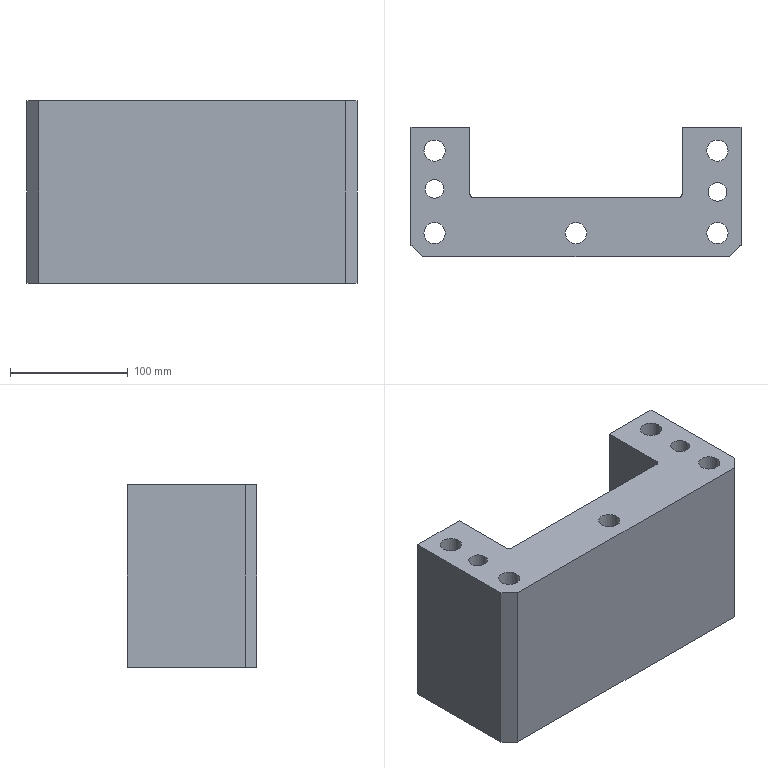Part | NX | features FD 2 | 1 solid | 47 faces | box 280 x 110 x 155 mm | volume 2587040 mm3 | plane 23 | cylinder 22 | cone 2 | commonest cylinder face diameters 18 x5 26 x5 21 x4 6 x2 14.1 x2 16.001 x2
STEP:
#1=CARTESIAN_POINT('',(2683.,562.5,256.5));
#2=VERTEX_POINT('',#1);
#3=CARTESIAN_POINT('',(2943.,562.5,256.5));
#4=VERTEX_POINT('',#3);
#5=CARTESIAN_POINT('',(2738.,562.5,256.5));
#6=DIRECTION('',(1.,0.,0.));
#7=VECTOR('',#6,1000.);
#8=LINE('',#5,#7);
#9=EDGE_CURVE('',#2,#4,#8,.T.);
#10=ORIENTED_EDGE('',*,*,#9,.F.);
#11=CARTESIAN_POINT('',(2683.,562.5,101.5));
#12=VERTEX_POINT('',#11);
#13=CARTESIAN_POINT('',(2683.,562.5,101.5));
#14=DIRECTION('',(0.,0.,-1.));
#15=VECTOR('',#14,1000.);
#16=LINE('',#13,#15);
#17=EDGE_CURVE('',#2,#12,#16,.T.);
#18=ORIENTED_EDGE('',*,*,#17,.T.);
#19=CARTESIAN_POINT('',(2943.,562.5,101.5));
#20=VERTEX_POINT('',#19);
#21=CARTESIAN_POINT('',(2738.,562.5,101.5));
#22=DIRECTION('',(1.,0.,0.));
#23=VECTOR('',#22,1000.);
#24=LINE('',#21,#23);
#25=EDGE_CURVE('',#12,#20,#24,.T.);
#26=ORIENTED_EDGE('',*,*,#25,.T.);
#27=CARTESIAN_POINT('',(2943.,562.5,191.5));
#28=DIRECTION('',(0.,0.,1.));
#29=VECTOR('',#28,1000.);
#30=LINE('',#27,#29);
#31=EDGE_CURVE('',#20,#4,#30,.T.);
#32=ORIENTED_EDGE('',*,*,#31,.T.);
#33=EDGE_LOOP('',(#10,#18,#26,#32));
#34=FACE_BOUND('',#33,.T.);
#35=CARTESIAN_POINT('',(2738.,562.5,191.5));
#36=DIRECTION('',(0.,1.,0.));
#37=DIRECTION('',(1.,0.,0.));
#38=AXIS2_PLACEMENT_3D('',#35,#36,#37);
#39=PLANE('',#38);
#40=ADVANCED_FACE('',(#34),#39,.F.);
#41=CARTESIAN_POINT('',(2953.,572.5,256.5));
#42=VERTEX_POINT('',#41);
#43=CARTESIAN_POINT('',(2953.,672.5,256.5));
#44=VERTEX_POINT('',#43);
#45=CARTESIAN_POINT('',(2953.,622.5,256.5));
#46=DIRECTION('',(0.,1.,0.));
#47=VECTOR('',#46,1000.);
#48=LINE('',#45,#47);
#49=EDGE_CURVE('',#42,#44,#48,.T.);
#50=ORIENTED_EDGE('',*,*,#49,.F.);
#51=CARTESIAN_POINT('',(2953.,572.5,101.5));
#52=VERTEX_POINT('',#51);
#53=CARTESIAN_POINT('',(2953.,572.5,191.5));
#54=DIRECTION('',(0.,0.,-1.));
#55=VECTOR('',#54,1000.);
#56=LINE('',#53,#55);
#57=EDGE_CURVE('',#42,#52,#56,.T.);
#58=ORIENTED_EDGE('',*,*,#57,.T.);
#59=CARTESIAN_POINT('',(2953.,672.5,101.5));
#60=VERTEX_POINT('',#59);
#61=CARTESIAN_POINT('',(2953.,622.5,101.5));
#62=DIRECTION('',(0.,1.,0.));
#63=VECTOR('',#62,1000.);
#64=LINE('',#61,#63);
#65=EDGE_CURVE('',#52,#60,#64,.T.);
#66=ORIENTED_EDGE('',*,*,#65,.T.);
#67=CARTESIAN_POINT('',(2953.,672.5,191.5));
#68=DIRECTION('',(0.,0.,1.));
#69=VECTOR('',#68,1000.);
#70=LINE('',#67,#69);
#71=EDGE_CURVE('',#60,#44,#70,.T.);
#72=ORIENTED_EDGE('',*,*,#71,.T.);
#73=EDGE_LOOP('',(#50,#58,#66,#72));
#74=FACE_BOUND('',#73,.T.);
#75=CARTESIAN_POINT('',(2953.,622.5,191.5));
#76=DIRECTION('',(-1.,0.,0.));
#77=DIRECTION('',(0.,1.,0.));
#78=AXIS2_PLACEMENT_3D('',#75,#76,#77);
#79=PLANE('',#78);
#80=ADVANCED_FACE('',(#74),#79,.F.);
#81=ORIENTED_EDGE('',*,*,#71,.F.);
#82=CARTESIAN_POINT('',(2903.,672.5,101.5));
#83=VERTEX_POINT('',#82);
#84=CARTESIAN_POINT('',(2918.,672.5,101.5));
#85=DIRECTION('',(1.,0.,0.));
#86=VECTOR('',#85,1000.);
#87=LINE('',#84,#86);
#88=EDGE_CURVE('',#83,#60,#87,.T.);
#89=ORIENTED_EDGE('',*,*,#88,.F.);
#90=CARTESIAN_POINT('',(2903.,672.5,256.5));
#91=VERTEX_POINT('',#90);
#92=CARTESIAN_POINT('',(2903.,672.5,191.5));
#93=DIRECTION('',(0.,0.,1.));
#94=VECTOR('',#93,1000.);
#95=LINE('',#92,#94);
#96=EDGE_CURVE('',#83,#91,#95,.T.);
#97=ORIENTED_EDGE('',*,*,#96,.T.);
#98=CARTESIAN_POINT('',(2918.,672.5,256.5));
#99=DIRECTION('',(1.,0.,0.));
#100=VECTOR('',#99,1000.);
#101=LINE('',#98,#100);
#102=EDGE_CURVE('',#91,#44,#101,.T.);
#103=ORIENTED_EDGE('',*,*,#102,.T.);
#104=EDGE_LOOP('',(#81,#89,#97,#103));
#105=FACE_BOUND('',#104,.T.);
#106=CARTESIAN_POINT('',(2918.,672.5,191.5));
#107=DIRECTION('',(0.,-1.,0.));
#108=DIRECTION('',(-1.,0.,0.));
#109=AXIS2_PLACEMENT_3D('',#106,#107,#108);
#110=PLANE('',#109);
#111=ADVANCED_FACE('',(#105),#110,.F.);
#112=CARTESIAN_POINT('',(2903.,615.5,101.5));
#113=VERTEX_POINT('',#112);
#114=CARTESIAN_POINT('',(2903.,622.5,101.5));
#115=DIRECTION('',(0.,1.,0.));
#116=VECTOR('',#115,1000.);
#117=LINE('',#114,#116);
#118=EDGE_CURVE('',#113,#83,#117,.T.);
#119=ORIENTED_EDGE('',*,*,#118,.F.);
#120=CARTESIAN_POINT('',(2903.,615.5,256.5));
#121=VERTEX_POINT('',#120);
#122=CARTESIAN_POINT('',(2903.,615.5,191.5));
#123=DIRECTION('',(0.,0.,1.));
#124=VECTOR('',#123,1000.);
#125=LINE('',#122,#124);
#126=EDGE_CURVE('',#113,#121,#125,.T.);
#127=ORIENTED_EDGE('',*,*,#126,.T.);
#128=CARTESIAN_POINT('',(2903.,622.5,256.5));
#129=DIRECTION('',(0.,1.,0.));
#130=VECTOR('',#129,1000.);
#131=LINE('',#128,#130);
#132=EDGE_CURVE('',#121,#91,#131,.T.);
#133=ORIENTED_EDGE('',*,*,#132,.T.);
#134=ORIENTED_EDGE('',*,*,#96,.F.);
#135=EDGE_LOOP('',(#119,#127,#133,#134));
#136=FACE_BOUND('',#135,.T.);
#137=CARTESIAN_POINT('',(2903.,622.5,191.5));
#138=DIRECTION('',(1.,0.,0.));
#139=DIRECTION('',(0.,-1.,0.));
#140=AXIS2_PLACEMENT_3D('',#137,#138,#139);
#141=PLANE('',#140);
#142=ADVANCED_FACE('',(#136),#141,.F.);
#143=CARTESIAN_POINT('',(2900.,612.5,101.5));
#144=VERTEX_POINT('',#143);
#145=CARTESIAN_POINT('',(2900.,615.5,101.5));
#146=DIRECTION('',(0.,0.,1.));
#147=DIRECTION('',(-1.,0.,0.));
#148=AXIS2_PLACEMENT_3D('',#145,#146,#147);
#149=CIRCLE('',#148,3.);
#150=EDGE_CURVE('',#144,#113,#149,.T.);
#151=ORIENTED_EDGE('',*,*,#150,.F.);
#152=CARTESIAN_POINT('',(2900.,612.5,256.5));
#153=VERTEX_POINT('',#152);
#154=CARTESIAN_POINT('',(2900.,612.5,191.5));
#155=DIRECTION('',(0.,0.,-1.));
#156=VECTOR('',#155,1000.);
#157=LINE('',#154,#156);
#158=EDGE_CURVE('',#153,#144,#157,.T.);
#159=ORIENTED_EDGE('',*,*,#158,.F.);
#160=CARTESIAN_POINT('',(2900.,615.5,256.5));
#161=DIRECTION('',(0.,0.,-1.));
#162=DIRECTION('',(1.,0.,0.));
#163=AXIS2_PLACEMENT_3D('',#160,#161,#162);
#164=CIRCLE('',#163,3.);
#165=EDGE_CURVE('',#121,#153,#164,.T.);
#166=ORIENTED_EDGE('',*,*,#165,.F.);
#167=ORIENTED_EDGE('',*,*,#126,.F.);
#168=EDGE_LOOP('',(#151,#159,#166,#167));
#169=FACE_BOUND('',#168,.T.);
#170=CARTESIAN_POINT('',(2900.,615.5,191.5));
#171=DIRECTION('',(0.,0.,-1.));
#172=DIRECTION('',(-1.,0.,0.));
#173=AXIS2_PLACEMENT_3D('',#170,#171,#172);
#174=CYLINDRICAL_SURFACE('',#173,3.);
#175=ADVANCED_FACE('',(#169),#174,.F.);
#176=CARTESIAN_POINT('',(2883.5,612.5,226.5));
#177=VERTEX_POINT('',#176);
#178=CARTESIAN_POINT('',(2873.,612.5,226.5));
#179=DIRECTION('',(0.,-1.,0.));
#180=DIRECTION('',(1.,0.,0.));
#181=AXIS2_PLACEMENT_3D('',#178,#179,#180);
#182=CIRCLE('',#181,10.5);
#183=EDGE_CURVE('',#177,#177,#182,.T.);
#184=ORIENTED_EDGE('',*,*,#183,.T.);
#185=EDGE_LOOP('',(#184));
#186=FACE_BOUND('',#185,.T.);
#187=CARTESIAN_POINT('',(2763.5,612.5,226.5));
#188=VERTEX_POINT('',#187);
#189=CARTESIAN_POINT('',(2753.,612.5,226.5));
#190=DIRECTION('',(0.,-1.,0.));
#191=DIRECTION('',(1.,0.,0.));
#192=AXIS2_PLACEMENT_3D('',#189,#190,#191);
#193=CIRCLE('',#192,10.5);
#194=EDGE_CURVE('',#188,#188,#193,.T.);
#195=ORIENTED_EDGE('',*,*,#194,.T.);
#196=EDGE_LOOP('',(#195));
#197=FACE_BOUND('',#196,.T.);
#198=CARTESIAN_POINT('',(2763.5,612.5,134.));
#199=VERTEX_POINT('',#198);
#200=CARTESIAN_POINT('',(2753.,612.5,134.));
#201=DIRECTION('',(0.,-1.,0.));
#202=DIRECTION('',(1.,0.,0.));
#203=AXIS2_PLACEMENT_3D('',#200,#201,#202);
#204=CIRCLE('',#203,10.5);
#205=EDGE_CURVE('',#199,#199,#204,.T.);
#206=ORIENTED_EDGE('',*,*,#205,.T.);
#207=EDGE_LOOP('',(#206));
#208=FACE_BOUND('',#207,.T.);
#209=CARTESIAN_POINT('',(2883.5,612.5,134.));
#210=VERTEX_POINT('',#209);
#211=CARTESIAN_POINT('',(2873.,612.5,134.));
#212=DIRECTION('',(0.,-1.,0.));
#213=DIRECTION('',(1.,0.,0.));
#214=AXIS2_PLACEMENT_3D('',#211,#212,#213);
#215=CIRCLE('',#214,10.5);
#216=EDGE_CURVE('',#210,#210,#215,.T.);
#217=ORIENTED_EDGE('',*,*,#216,.T.);
#218=EDGE_LOOP('',(#217));
#219=FACE_BOUND('',#218,.T.);
#220=CARTESIAN_POINT('',(2726.,612.5,101.5));
#221=VERTEX_POINT('',#220);
#222=CARTESIAN_POINT('',(2738.,612.5,101.5));
#223=DIRECTION('',(1.,0.,0.));
#224=VECTOR('',#223,1000.);
#225=LINE('',#222,#224);
#226=EDGE_CURVE('',#221,#144,#225,.T.);
#227=ORIENTED_EDGE('',*,*,#226,.F.);
#228=CARTESIAN_POINT('',(2726.,612.5,256.5));
#229=VERTEX_POINT('',#228);
#230=CARTESIAN_POINT('',(2726.,612.5,191.5));
#231=DIRECTION('',(0.,0.,1.));
#232=VECTOR('',#231,1000.);
#233=LINE('',#230,#232);
#234=EDGE_CURVE('',#221,#229,#233,.T.);
#235=ORIENTED_EDGE('',*,*,#234,.T.);
#236=CARTESIAN_POINT('',(2738.,612.5,256.5));
#237=DIRECTION('',(1.,0.,0.));
#238=VECTOR('',#237,1000.);
#239=LINE('',#236,#238);
#240=EDGE_CURVE('',#229,#153,#239,.T.);
#241=ORIENTED_EDGE('',*,*,#240,.T.);
#242=ORIENTED_EDGE('',*,*,#158,.T.);
#243=EDGE_LOOP('',(#227,#235,#241,#242));
#244=FACE_BOUND('',#243,.T.);
#245=CARTESIAN_POINT('',(2738.,612.5,191.5));
#246=DIRECTION('',(0.,-1.,0.));
#247=DIRECTION('',(-1.,0.,0.));
#248=AXIS2_PLACEMENT_3D('',#245,#246,#247);
#249=PLANE('',#248);
#250=ADVANCED_FACE('',(#186,#197,#208,#219,#244),#249,.F.);
#251=CARTESIAN_POINT('',(2723.,615.5,101.5));
#252=VERTEX_POINT('',#251);
#253=CARTESIAN_POINT('',(2726.,615.5,101.5));
#254=DIRECTION('',(0.,0.,1.));
#255=DIRECTION('',(-1.,0.,0.));
#256=AXIS2_PLACEMENT_3D('',#253,#254,#255);
#257=CIRCLE('',#256,3.);
#258=EDGE_CURVE('',#252,#221,#257,.T.);
#259=ORIENTED_EDGE('',*,*,#258,.F.);
#260=CARTESIAN_POINT('',(2723.,615.5,256.5));
#261=VERTEX_POINT('',#260);
#262=CARTESIAN_POINT('',(2723.,615.5,191.5));
#263=DIRECTION('',(0.,0.,-1.));
#264=VECTOR('',#263,1000.);
#265=LINE('',#262,#264);
#266=EDGE_CURVE('',#261,#252,#265,.T.);
#267=ORIENTED_EDGE('',*,*,#266,.F.);
#268=CARTESIAN_POINT('',(2726.,615.5,256.5));
#269=DIRECTION('',(0.,0.,-1.));
#270=DIRECTION('',(1.,0.,0.));
#271=AXIS2_PLACEMENT_3D('',#268,#269,#270);
#272=CIRCLE('',#271,3.);
#273=EDGE_CURVE('',#229,#261,#272,.T.);
#274=ORIENTED_EDGE('',*,*,#273,.F.);
#275=ORIENTED_EDGE('',*,*,#234,.F.);
#276=EDGE_LOOP('',(#259,#267,#274,#275));
#277=FACE_BOUND('',#276,.T.);
#278=CARTESIAN_POINT('',(2726.,615.5,191.5));
#279=DIRECTION('',(0.,0.,-1.));
#280=DIRECTION('',(-1.,0.,0.));
#281=AXIS2_PLACEMENT_3D('',#278,#279,#280);
#282=CYLINDRICAL_SURFACE('',#281,3.);
#283=ADVANCED_FACE('',(#277),#282,.F.);
#284=CARTESIAN_POINT('',(2723.,672.5,256.5));
#285=VERTEX_POINT('',#284);
#286=CARTESIAN_POINT('',(2723.,667.5,256.5));
#287=DIRECTION('',(0.,-1.,0.));
#288=VECTOR('',#287,1000.);
#289=LINE('',#286,#288);
#290=EDGE_CURVE('',#285,#261,#289,.T.);
#291=ORIENTED_EDGE('',*,*,#290,.T.);
#292=ORIENTED_EDGE('',*,*,#266,.T.);
#293=CARTESIAN_POINT('',(2723.,672.5,101.5));
#294=VERTEX_POINT('',#293);
#295=CARTESIAN_POINT('',(2723.,667.5,101.5));
#296=DIRECTION('',(0.,-1.,0.));
#297=VECTOR('',#296,1000.);
#298=LINE('',#295,#297);
#299=EDGE_CURVE('',#294,#252,#298,.T.);
#300=ORIENTED_EDGE('',*,*,#299,.F.);
#301=CARTESIAN_POINT('',(2723.,672.5,191.5));
#302=DIRECTION('',(0.,0.,1.));
#303=VECTOR('',#302,1000.);
#304=LINE('',#301,#303);
#305=EDGE_CURVE('',#294,#285,#304,.T.);
#306=ORIENTED_EDGE('',*,*,#305,.T.);
#307=EDGE_LOOP('',(#291,#292,#300,#306));
#308=FACE_BOUND('',#307,.T.);
#309=CARTESIAN_POINT('',(2723.,667.5,191.5));
#310=DIRECTION('',(-1.,0.,0.));
#311=DIRECTION('',(0.,1.,0.));
#312=AXIS2_PLACEMENT_3D('',#309,#310,#311);
#313=PLANE('',#312);
#314=ADVANCED_FACE('',(#308),#313,.F.);
#315=ORIENTED_EDGE('',*,*,#305,.F.);
#316=CARTESIAN_POINT('',(2673.,672.5,101.5));
#317=VERTEX_POINT('',#316);
#318=CARTESIAN_POINT('',(2708.,672.5,101.5));
#319=DIRECTION('',(-1.,0.,0.));
#320=VECTOR('',#319,1000.);
#321=LINE('',#318,#320);
#322=EDGE_CURVE('',#294,#317,#321,.T.);
#323=ORIENTED_EDGE('',*,*,#322,.T.);
#324=CARTESIAN_POINT('',(2673.,672.5,256.5));
#325=VERTEX_POINT('',#324);
#326=CARTESIAN_POINT('',(2673.,672.5,191.5));
#327=DIRECTION('',(0.,0.,1.));
#328=VECTOR('',#327,1000.);
#329=LINE('',#326,#328);
#330=EDGE_CURVE('',#317,#325,#329,.T.);
#331=ORIENTED_EDGE('',*,*,#330,.T.);
#332=CARTESIAN_POINT('',(2708.,672.5,256.5));
#333=DIRECTION('',(-1.,0.,0.));
#334=VECTOR('',#333,1000.);
#335=LINE('',#332,#334);
#336=EDGE_CURVE('',#285,#325,#335,.T.);
#337=ORIENTED_EDGE('',*,*,#336,.F.);
#338=EDGE_LOOP('',(#315,#323,#331,#337));
#339=FACE_BOUND('',#338,.T.);
#340=CARTESIAN_POINT('',(2708.,672.5,191.5));
#341=DIRECTION('',(0.,1.,0.));
#342=DIRECTION('',(1.,0.,0.));
#343=AXIS2_PLACEMENT_3D('',#340,#341,#342);
#344=PLANE('',#343);
#345=ADVANCED_FACE('',(#339),#344,.T.);
#346=CARTESIAN_POINT('',(2673.,572.5,101.5));
#347=VERTEX_POINT('',#346);
#348=CARTESIAN_POINT('',(2673.,667.5,101.5));
#349=DIRECTION('',(0.,-1.,0.));
#350=VECTOR('',#349,1000.);
#351=LINE('',#348,#350);
#352=EDGE_CURVE('',#317,#347,#351,.T.);
#353=ORIENTED_EDGE('',*,*,#352,.T.);
#354=CARTESIAN_POINT('',(2673.,572.5,256.5));
#355=VERTEX_POINT('',#354);
#356=CARTESIAN_POINT('',(2673.,572.5,276.5));
#357=DIRECTION('',(0.,0.,1.));
#358=VECTOR('',#357,1000.);
#359=LINE('',#356,#358);
#360=EDGE_CURVE('',#347,#355,#359,.T.);
#361=ORIENTED_EDGE('',*,*,#360,.T.);
#362=CARTESIAN_POINT('',(2673.,667.5,256.5));
#363=DIRECTION('',(0.,-1.,0.));
#364=VECTOR('',#363,1000.);
#365=LINE('',#362,#364);
#366=EDGE_CURVE('',#325,#355,#365,.T.);
#367=ORIENTED_EDGE('',*,*,#366,.F.);
#368=ORIENTED_EDGE('',*,*,#330,.F.);
#369=EDGE_LOOP('',(#353,#361,#367,#368));
#370=FACE_BOUND('',#369,.T.);
#371=CARTESIAN_POINT('',(2673.,667.5,191.5));
#372=DIRECTION('',(-1.,0.,0.));
#373=DIRECTION('',(0.,1.,0.));
#374=AXIS2_PLACEMENT_3D('',#371,#372,#373);
#375=PLANE('',#374);
#376=ADVANCED_FACE('',(#370),#375,.T.);
#377=CARTESIAN_POINT('',(2701.001,620.,256.5));
#378=VERTEX_POINT('',#377);
#379=CARTESIAN_POINT('',(2693.,620.,256.5));
#380=DIRECTION('',(0.,0.,-1.));
#381=DIRECTION('',(1.,0.,0.));
#382=AXIS2_PLACEMENT_3D('',#379,#380,#381);
#383=CIRCLE('',#382,8.001);
#384=EDGE_CURVE('',#378,#378,#383,.T.);
#385=ORIENTED_EDGE('',*,*,#384,.T.);
#386=EDGE_LOOP('',(#385));
#387=FACE_BOUND('',#386,.T.);
#388=CARTESIAN_POINT('',(2941.001,617.5,256.5));
#389=VERTEX_POINT('',#388);
#390=CARTESIAN_POINT('',(2933.,617.5,256.5));
#391=DIRECTION('',(0.,0.,-1.));
#392=DIRECTION('',(1.,0.,0.));
#393=AXIS2_PLACEMENT_3D('',#390,#391,#392);
#394=CIRCLE('',#393,8.001);
#395=EDGE_CURVE('',#389,#389,#394,.T.);
#396=ORIENTED_EDGE('',*,*,#395,.T.);
#397=EDGE_LOOP('',(#396));
#398=FACE_BOUND('',#397,.T.);
#399=CARTESIAN_POINT('',(2822.,582.5,256.5));
#400=VERTEX_POINT('',#399);
#401=CARTESIAN_POINT('',(2813.,582.5,256.5));
#402=DIRECTION('',(0.,0.,-1.));
#403=DIRECTION('',(1.,0.,0.));
#404=AXIS2_PLACEMENT_3D('',#401,#402,#403);
#405=CIRCLE('',#404,9.);
#406=EDGE_CURVE('',#400,#400,#405,.T.);
#407=ORIENTED_EDGE('',*,*,#406,.T.);
#408=EDGE_LOOP('',(#407));
#409=FACE_BOUND('',#408,.T.);
#410=CARTESIAN_POINT('',(2942.,652.5,256.5));
#411=VERTEX_POINT('',#410);
#412=CARTESIAN_POINT('',(2933.,652.5,256.5));
#413=DIRECTION('',(0.,0.,-1.));
#414=DIRECTION('',(1.,0.,0.));
#415=AXIS2_PLACEMENT_3D('',#412,#413,#414);
#416=CIRCLE('',#415,9.);
#417=EDGE_CURVE('',#411,#411,#416,.T.);
#418=ORIENTED_EDGE('',*,*,#417,.T.);
#419=EDGE_LOOP('',(#418));
#420=FACE_BOUND('',#419,.T.);
#421=CARTESIAN_POINT('',(2702.,582.5,256.5));
#422=VERTEX_POINT('',#421);
#423=CARTESIAN_POINT('',(2693.,582.5,256.5));
#424=DIRECTION('',(0.,0.,-1.));
#425=DIRECTION('',(1.,0.,0.));
#426=AXIS2_PLACEMENT_3D('',#423,#424,#425);
#427=CIRCLE('',#426,9.);
#428=EDGE_CURVE('',#422,#422,#427,.T.);
#429=ORIENTED_EDGE('',*,*,#428,.T.);
#430=EDGE_LOOP('',(#429));
#431=FACE_BOUND('',#430,.T.);
#432=CARTESIAN_POINT('',(2702.,652.5,256.5));
#433=VERTEX_POINT('',#432);
#434=CARTESIAN_POINT('',(2693.,652.5,256.5));
#435=DIRECTION('',(0.,0.,-1.));
#436=DIRECTION('',(1.,0.,0.));
#437=AXIS2_PLACEMENT_3D('',#434,#435,#436);
#438=CIRCLE('',#437,9.);
#439=EDGE_CURVE('',#433,#433,#438,.T.);
#440=ORIENTED_EDGE('',*,*,#439,.T.);
#441=EDGE_LOOP('',(#440));
#442=FACE_BOUND('',#441,.T.);
#443=CARTESIAN_POINT('',(2942.,582.5,256.5));
#444=VERTEX_POINT('',#443);
#445=CARTESIAN_POINT('',(2933.,582.5,256.5));
#446=DIRECTION('',(0.,0.,-1.));
#447=DIRECTION('',(1.,0.,0.));
#448=AXIS2_PLACEMENT_3D('',#445,#446,#447);
#449=CIRCLE('',#448,9.);
#450=EDGE_CURVE('',#444,#444,#449,.T.);
#451=ORIENTED_EDGE('',*,*,#450,.T.);
#452=EDGE_LOOP('',(#451));
#453=FACE_BOUND('',#452,.T.);
#454=ORIENTED_EDGE('',*,*,#366,.T.);
#455=CARTESIAN_POINT('',(2658.,587.5,256.5));
#456=DIRECTION('',(0.7071,-0.7071,0.));
#457=VECTOR('',#456,1000.);
#458=LINE('',#455,#457);
#459=EDGE_CURVE('',#355,#2,#458,.T.);
#460=ORIENTED_EDGE('',*,*,#459,.T.);
#461=ORIENTED_EDGE('',*,*,#9,.T.);
#462=CARTESIAN_POINT('',(2893.,512.5,256.5));
#463=DIRECTION('',(0.7071,0.7071,0.));
#464=VECTOR('',#463,1000.);
#465=LINE('',#462,#464);
#466=EDGE_CURVE('',#4,#42,#465,.T.);
#467=ORIENTED_EDGE('',*,*,#466,.T.);
#468=ORIENTED_EDGE('',*,*,#49,.T.);
#469=ORIENTED_EDGE('',*,*,#102,.F.);
#470=ORIENTED_EDGE('',*,*,#132,.F.);
#471=ORIENTED_EDGE('',*,*,#165,.T.);
#472=ORIENTED_EDGE('',*,*,#240,.F.);
#473=ORIENTED_EDGE('',*,*,#273,.T.);
#474=ORIENTED_EDGE('',*,*,#290,.F.);
#475=ORIENTED_EDGE('',*,*,#336,.T.);
#476=EDGE_LOOP('',(#454,#460,#461,#467,#468,#469,#470,#471,#472,#473,#474,#475));
#477=FACE_BOUND('',#476,.T.);
#478=CARTESIAN_POINT('',(2738.,667.5,256.5));
#479=DIRECTION('',(0.,0.,1.));
#480=DIRECTION('',(0.,1.,0.));
#481=AXIS2_PLACEMENT_3D('',#478,#479,#480);
#482=PLANE('',#481);
#483=ADVANCED_FACE('',(#387,#398,#409,#420,#431,#442,#453,#477),#482,.T.);
#484=ORIENTED_EDGE('',*,*,#450,.F.);
#485=EDGE_LOOP('',(#484));
#486=FACE_BOUND('',#485,.T.);
#487=CARTESIAN_POINT('',(2942.,582.5,216.5));
#488=VERTEX_POINT('',#487);
#489=CARTESIAN_POINT('',(2933.,582.5,216.5));
#490=DIRECTION('',(0.,0.,-1.));
#491=DIRECTION('',(1.,0.,0.));
#492=AXIS2_PLACEMENT_3D('',#489,#490,#491);
#493=CIRCLE('',#492,9.);
#494=EDGE_CURVE('',#488,#488,#493,.T.);
#495=ORIENTED_EDGE('',*,*,#494,.T.);
#496=EDGE_LOOP('',(#495));
#497=FACE_BOUND('',#496,.T.);
#498=CARTESIAN_POINT('',(2933.,582.5,101.5));
#499=DIRECTION('',(0.,0.,1.));
#500=DIRECTION('',(1.,0.,0.));
#501=AXIS2_PLACEMENT_3D('',#498,#499,#500);
#502=CYLINDRICAL_SURFACE('',#501,9.);
#503=ADVANCED_FACE('',(#486,#497),#502,.F.);
#504=ORIENTED_EDGE('',*,*,#494,.F.);
#505=EDGE_LOOP('',(#504));
#506=FACE_BOUND('',#505,.T.);
#507=CARTESIAN_POINT('',(2946.,582.5,216.5));
#508=VERTEX_POINT('',#507);
#509=CARTESIAN_POINT('',(2933.,582.5,216.5));
#510=DIRECTION('',(0.,0.,-1.));
#511=DIRECTION('',(1.,0.,0.));
#512=AXIS2_PLACEMENT_3D('',#509,#510,#511);
#513=CIRCLE('',#512,13.);
#514=EDGE_CURVE('',#508,#508,#513,.T.);
#515=ORIENTED_EDGE('',*,*,#514,.T.);
#516=EDGE_LOOP('',(#515));
#517=FACE_BOUND('',#516,.T.);
#518=CARTESIAN_POINT('',(2933.,582.5,216.5));
#519=DIRECTION('',(0.,0.,1.));
#520=DIRECTION('',(1.,0.,0.));
#521=AXIS2_PLACEMENT_3D('',#518,#519,#520);
#522=PLANE('',#521);
#523=ADVANCED_FACE('',(#506,#517),#522,.F.);
#524=ORIENTED_EDGE('',*,*,#514,.F.);
#525=EDGE_LOOP('',(#524));
#526=FACE_BOUND('',#525,.T.);
#527=CARTESIAN_POINT('',(2946.,582.5,101.5));
#528=VERTEX_POINT('',#527);
#529=CARTESIAN_POINT('',(2933.,582.5,101.5));
#530=DIRECTION('',(0.,0.,-1.));
#531=DIRECTION('',(1.,0.,0.));
#532=AXIS2_PLACEMENT_3D('',#529,#530,#531);
#533=CIRCLE('',#532,13.);
#534=EDGE_CURVE('',#528,#528,#533,.T.);
#535=ORIENTED_EDGE('',*,*,#534,.T.);
#536=EDGE_LOOP('',(#535));
#537=FACE_BOUND('',#536,.T.);
#538=CARTESIAN_POINT('',(2933.,582.5,126.5));
#539=DIRECTION('',(0.,0.,1.));
#540=DIRECTION('',(1.,0.,0.));
#541=AXIS2_PLACEMENT_3D('',#538,#539,#540);
#542=CYLINDRICAL_SURFACE('',#541,13.);
#543=ADVANCED_FACE('',(#526,#537),#542,.F.);
#544=ORIENTED_EDGE('',*,*,#439,.F.);
#545=EDGE_LOOP('',(#544));
#546=FACE_BOUND('',#545,.T.);
#547=CARTESIAN_POINT('',(2702.,652.5,216.5));
#548=VERTEX_POINT('',#547);
#549=CARTESIAN_POINT('',(2693.,652.5,216.5));
#550=DIRECTION('',(0.,0.,-1.));
#551=DIRECTION('',(1.,0.,0.));
#552=AXIS2_PLACEMENT_3D('',#549,#550,#551);
#553=CIRCLE('',#552,9.);
#554=EDGE_CURVE('',#548,#548,#553,.T.);
#555=ORIENTED_EDGE('',*,*,#554,.T.);
#556=EDGE_LOOP('',(#555));
#557=FACE_BOUND('',#556,.T.);
#558=CARTESIAN_POINT('',(2693.,652.5,101.5));
#559=DIRECTION('',(0.,0.,1.));
#560=DIRECTION('',(1.,0.,0.));
#561=AXIS2_PLACEMENT_3D('',#558,#559,#560);
#562=CYLINDRICAL_SURFACE('',#561,9.);
#563=ADVANCED_FACE('',(#546,#557),#562,.F.);
#564=ORIENTED_EDGE('',*,*,#554,.F.);
#565=EDGE_LOOP('',(#564));
#566=FACE_BOUND('',#565,.T.);
#567=CARTESIAN_POINT('',(2706.,652.5,216.5));
#568=VERTEX_POINT('',#567);
#569=CARTESIAN_POINT('',(2693.,652.5,216.5));
#570=DIRECTION('',(0.,0.,-1.));
#571=DIRECTION('',(1.,0.,0.));
#572=AXIS2_PLACEMENT_3D('',#569,#570,#571);
#573=CIRCLE('',#572,13.);
#574=EDGE_CURVE('',#568,#568,#573,.T.);
#575=ORIENTED_EDGE('',*,*,#574,.T.);
#576=EDGE_LOOP('',(#575));
#577=FACE_BOUND('',#576,.T.);
#578=CARTESIAN_POINT('',(2693.,652.5,216.5));
#579=DIRECTION('',(0.,0.,1.));
#580=DIRECTION('',(1.,0.,0.));
#581=AXIS2_PLACEMENT_3D('',#578,#579,#580);
#582=PLANE('',#581);
#583=ADVANCED_FACE('',(#566,#577),#582,.F.);
#584=ORIENTED_EDGE('',*,*,#574,.F.);
#585=EDGE_LOOP('',(#584));
#586=FACE_BOUND('',#585,.T.);
#587=CARTESIAN_POINT('',(2706.,652.5,101.5));
#588=VERTEX_POINT('',#587);
#589=CARTESIAN_POINT('',(2693.,652.5,101.5));
#590=DIRECTION('',(0.,0.,-1.));
#591=DIRECTION('',(1.,0.,0.));
#592=AXIS2_PLACEMENT_3D('',#589,#590,#591);
#593=CIRCLE('',#592,13.);
#594=EDGE_CURVE('',#588,#588,#593,.T.);
#595=ORIENTED_EDGE('',*,*,#594,.T.);
#596=EDGE_LOOP('',(#595));
#597=FACE_BOUND('',#596,.T.);
#598=CARTESIAN_POINT('',(2693.,652.5,126.5));
#599=DIRECTION('',(0.,0.,1.));
#600=DIRECTION('',(1.,0.,0.));
#601=AXIS2_PLACEMENT_3D('',#598,#599,#600);
#602=CYLINDRICAL_SURFACE('',#601,13.);
#603=ADVANCED_FACE('',(#586,#597),#602,.F.);
#604=ORIENTED_EDGE('',*,*,#428,.F.);
#605=EDGE_LOOP('',(#604));
#606=FACE_BOUND('',#605,.T.);
#607=CARTESIAN_POINT('',(2702.,582.5,216.5));
#608=VERTEX_POINT('',#607);
#609=CARTESIAN_POINT('',(2693.,582.5,216.5));
#610=DIRECTION('',(0.,0.,-1.));
#611=DIRECTION('',(1.,0.,0.));
#612=AXIS2_PLACEMENT_3D('',#609,#610,#611);
#613=CIRCLE('',#612,9.);
#614=EDGE_CURVE('',#608,#608,#613,.T.);
#615=ORIENTED_EDGE('',*,*,#614,.T.);
#616=EDGE_LOOP('',(#615));
#617=FACE_BOUND('',#616,.T.);
#618=CARTESIAN_POINT('',(2693.,582.5,101.5));
#619=DIRECTION('',(0.,0.,1.));
#620=DIRECTION('',(1.,0.,0.));
#621=AXIS2_PLACEMENT_3D('',#618,#619,#620);
#622=CYLINDRICAL_SURFACE('',#621,9.);
#623=ADVANCED_FACE('',(#606,#617),#622,.F.);
#624=ORIENTED_EDGE('',*,*,#614,.F.);
#625=EDGE_LOOP('',(#624));
#626=FACE_BOUND('',#625,.T.);
#627=CARTESIAN_POINT('',(2706.,582.5,216.5));
#628=VERTEX_POINT('',#627);
#629=CARTESIAN_POINT('',(2693.,582.5,216.5));
#630=DIRECTION('',(0.,0.,-1.));
#631=DIRECTION('',(1.,0.,0.));
#632=AXIS2_PLACEMENT_3D('',#629,#630,#631);
#633=CIRCLE('',#632,13.);
#634=EDGE_CURVE('',#628,#628,#633,.T.);
#635=ORIENTED_EDGE('',*,*,#634,.T.);
#636=EDGE_LOOP('',(#635));
#637=FACE_BOUND('',#636,.T.);
#638=CARTESIAN_POINT('',(2693.,582.5,216.5));
#639=DIRECTION('',(0.,0.,1.));
#640=DIRECTION('',(1.,0.,0.));
#641=AXIS2_PLACEMENT_3D('',#638,#639,#640);
#642=PLANE('',#641);
#643=ADVANCED_FACE('',(#626,#637),#642,.F.);
#644=ORIENTED_EDGE('',*,*,#634,.F.);
#645=EDGE_LOOP('',(#644));
#646=FACE_BOUND('',#645,.T.);
#647=CARTESIAN_POINT('',(2706.,582.5,101.5));
#648=VERTEX_POINT('',#647);
#649=CARTESIAN_POINT('',(2693.,582.5,101.5));
#650=DIRECTION('',(0.,0.,-1.));
#651=DIRECTION('',(1.,0.,0.));
#652=AXIS2_PLACEMENT_3D('',#649,#650,#651);
#653=CIRCLE('',#652,13.);
#654=EDGE_CURVE('',#648,#648,#653,.T.);
#655=ORIENTED_EDGE('',*,*,#654,.T.);
#656=EDGE_LOOP('',(#655));
#657=FACE_BOUND('',#656,.T.);
#658=CARTESIAN_POINT('',(2693.,582.5,126.5));
#659=DIRECTION('',(0.,0.,1.));
#660=DIRECTION('',(1.,0.,0.));
#661=AXIS2_PLACEMENT_3D('',#658,#659,#660);
#662=CYLINDRICAL_SURFACE('',#661,13.);
#663=ADVANCED_FACE('',(#646,#657),#662,.F.);
#664=ORIENTED_EDGE('',*,*,#417,.F.);
#665=EDGE_LOOP('',(#664));
#666=FACE_BOUND('',#665,.T.);
#667=CARTESIAN_POINT('',(2942.,652.5,216.5));
#668=VERTEX_POINT('',#667);
#669=CARTESIAN_POINT('',(2933.,652.5,216.5));
#670=DIRECTION('',(0.,0.,-1.));
#671=DIRECTION('',(1.,0.,0.));
#672=AXIS2_PLACEMENT_3D('',#669,#670,#671);
#673=CIRCLE('',#672,9.);
#674=EDGE_CURVE('',#668,#668,#673,.T.);
#675=ORIENTED_EDGE('',*,*,#674,.T.);
#676=EDGE_LOOP('',(#675));
#677=FACE_BOUND('',#676,.T.);
#678=CARTESIAN_POINT('',(2933.,652.5,101.5));
#679=DIRECTION('',(0.,0.,1.));
#680=DIRECTION('',(1.,0.,0.));
#681=AXIS2_PLACEMENT_3D('',#678,#679,#680);
#682=CYLINDRICAL_SURFACE('',#681,9.);
#683=ADVANCED_FACE('',(#666,#677),#682,.F.);
#684=ORIENTED_EDGE('',*,*,#674,.F.);
#685=EDGE_LOOP('',(#684));
#686=FACE_BOUND('',#685,.T.);
#687=CARTESIAN_POINT('',(2946.,652.5,216.5));
#688=VERTEX_POINT('',#687);
#689=CARTESIAN_POINT('',(2933.,652.5,216.5));
#690=DIRECTION('',(0.,0.,-1.));
#691=DIRECTION('',(1.,0.,0.));
#692=AXIS2_PLACEMENT_3D('',#689,#690,#691);
#693=CIRCLE('',#692,13.);
#694=EDGE_CURVE('',#688,#688,#693,.T.);
#695=ORIENTED_EDGE('',*,*,#694,.T.);
#696=EDGE_LOOP('',(#695));
#697=FACE_BOUND('',#696,.T.);
#698=CARTESIAN_POINT('',(2933.,652.5,216.5));
#699=DIRECTION('',(0.,0.,1.));
#700=DIRECTION('',(1.,0.,0.));
#701=AXIS2_PLACEMENT_3D('',#698,#699,#700);
#702=PLANE('',#701);
#703=ADVANCED_FACE('',(#686,#697),#702,.F.);
#704=ORIENTED_EDGE('',*,*,#694,.F.);
#705=EDGE_LOOP('',(#704));
#706=FACE_BOUND('',#705,.T.);
#707=CARTESIAN_POINT('',(2946.,652.5,101.5));
#708=VERTEX_POINT('',#707);
#709=CARTESIAN_POINT('',(2933.,652.5,101.5));
#710=DIRECTION('',(0.,0.,-1.));
#711=DIRECTION('',(1.,0.,0.));
#712=AXIS2_PLACEMENT_3D('',#709,#710,#711);
#713=CIRCLE('',#712,13.);
#714=EDGE_CURVE('',#708,#708,#713,.T.);
#715=ORIENTED_EDGE('',*,*,#714,.T.);
#716=EDGE_LOOP('',(#715));
#717=FACE_BOUND('',#716,.T.);
#718=CARTESIAN_POINT('',(2933.,652.5,126.5));
#719=DIRECTION('',(0.,0.,1.));
#720=DIRECTION('',(1.,0.,0.));
#721=AXIS2_PLACEMENT_3D('',#718,#719,#720);
#722=CYLINDRICAL_SURFACE('',#721,13.);
#723=ADVANCED_FACE('',(#706,#717),#722,.F.);
#724=ORIENTED_EDGE('',*,*,#406,.F.);
#725=EDGE_LOOP('',(#724));
#726=FACE_BOUND('',#725,.T.);
#727=CARTESIAN_POINT('',(2822.,582.5,216.5));
#728=VERTEX_POINT('',#727);
#729=CARTESIAN_POINT('',(2813.,582.5,216.5));
#730=DIRECTION('',(0.,0.,-1.));
#731=DIRECTION('',(1.,0.,0.));
#732=AXIS2_PLACEMENT_3D('',#729,#730,#731);
#733=CIRCLE('',#732,9.);
#734=EDGE_CURVE('',#728,#728,#733,.T.);
#735=ORIENTED_EDGE('',*,*,#734,.T.);
#736=EDGE_LOOP('',(#735));
#737=FACE_BOUND('',#736,.T.);
#738=CARTESIAN_POINT('',(2813.,582.5,101.5));
#739=DIRECTION('',(0.,0.,1.));
#740=DIRECTION('',(1.,0.,0.));
#741=AXIS2_PLACEMENT_3D('',#738,#739,#740);
#742=CYLINDRICAL_SURFACE('',#741,9.);
#743=ADVANCED_FACE('',(#726,#737),#742,.F.);
#744=ORIENTED_EDGE('',*,*,#734,.F.);
#745=EDGE_LOOP('',(#744));
#746=FACE_BOUND('',#745,.T.);
#747=CARTESIAN_POINT('',(2826.,582.5,216.5));
#748=VERTEX_POINT('',#747);
#749=CARTESIAN_POINT('',(2813.,582.5,216.5));
#750=DIRECTION('',(0.,0.,-1.));
#751=DIRECTION('',(1.,0.,0.));
#752=AXIS2_PLACEMENT_3D('',#749,#750,#751);
#753=CIRCLE('',#752,13.);
#754=EDGE_CURVE('',#748,#748,#753,.T.);
#755=ORIENTED_EDGE('',*,*,#754,.T.);
#756=EDGE_LOOP('',(#755));
#757=FACE_BOUND('',#756,.T.);
#758=CARTESIAN_POINT('',(2813.,582.5,216.5));
#759=DIRECTION('',(0.,0.,1.));
#760=DIRECTION('',(1.,0.,0.));
#761=AXIS2_PLACEMENT_3D('',#758,#759,#760);
#762=PLANE('',#761);
#763=ADVANCED_FACE('',(#746,#757),#762,.F.);
#764=ORIENTED_EDGE('',*,*,#754,.F.);
#765=EDGE_LOOP('',(#764));
#766=FACE_BOUND('',#765,.T.);
#767=CARTESIAN_POINT('',(2826.,582.5,101.5));
#768=VERTEX_POINT('',#767);
#769=CARTESIAN_POINT('',(2813.,582.5,101.5));
#770=DIRECTION('',(0.,0.,-1.));
#771=DIRECTION('',(1.,0.,0.));
#772=AXIS2_PLACEMENT_3D('',#769,#770,#771);
#773=CIRCLE('',#772,13.);
#774=EDGE_CURVE('',#768,#768,#773,.T.);
#775=ORIENTED_EDGE('',*,*,#774,.T.);
#776=EDGE_LOOP('',(#775));
#777=FACE_BOUND('',#776,.T.);
#778=CARTESIAN_POINT('',(2813.,582.5,126.5));
#779=DIRECTION('',(0.,0.,1.));
#780=DIRECTION('',(1.,0.,0.));
#781=AXIS2_PLACEMENT_3D('',#778,#779,#780);
#782=CYLINDRICAL_SURFACE('',#781,13.);
#783=ADVANCED_FACE('',(#766,#777),#782,.F.);
#784=CARTESIAN_POINT('',(2941.755,617.5,207.5));
#785=VERTEX_POINT('',#784);
#786=CARTESIAN_POINT('',(2933.,617.5,207.5));
#787=DIRECTION('',(0.,0.,-1.));
#788=DIRECTION('',(1.,0.,0.));
#789=AXIS2_PLACEMENT_3D('',#786,#787,#788);
#790=CIRCLE('',#789,8.755);
#791=EDGE_CURVE('',#785,#785,#790,.T.);
#792=ORIENTED_EDGE('',*,*,#791,.F.);
#793=EDGE_LOOP('',(#792));
#794=FACE_BOUND('',#793,.T.);
#795=CARTESIAN_POINT('',(2941.755,617.5,101.5));
#796=VERTEX_POINT('',#795);
#797=CARTESIAN_POINT('',(2933.,617.5,101.5));
#798=DIRECTION('',(0.,0.,-1.));
#799=DIRECTION('',(1.,0.,0.));
#800=AXIS2_PLACEMENT_3D('',#797,#798,#799);
#801=CIRCLE('',#800,8.755);
#802=EDGE_CURVE('',#796,#796,#801,.T.);
#803=ORIENTED_EDGE('',*,*,#802,.T.);
#804=EDGE_LOOP('',(#803));
#805=FACE_BOUND('',#804,.T.);
#806=CARTESIAN_POINT('',(2933.,617.5,121.5));
#807=DIRECTION('',(0.,0.,1.));
#808=DIRECTION('',(1.,0.,0.));
#809=AXIS2_PLACEMENT_3D('',#806,#807,#808);
#810=CYLINDRICAL_SURFACE('',#809,8.755);
#811=ADVANCED_FACE('',(#794,#805),#810,.F.);
#812=ORIENTED_EDGE('',*,*,#395,.F.);
#813=EDGE_LOOP('',(#812));
#814=FACE_BOUND('',#813,.T.);
#815=CARTESIAN_POINT('',(2941.001,617.5,207.5));
#816=VERTEX_POINT('',#815);
#817=CARTESIAN_POINT('',(2933.,617.5,207.5));
#818=DIRECTION('',(0.,0.,-1.));
#819=DIRECTION('',(1.,0.,0.));
#820=AXIS2_PLACEMENT_3D('',#817,#818,#819);
#821=CIRCLE('',#820,8.001);
#822=EDGE_CURVE('',#816,#816,#821,.T.);
#823=ORIENTED_EDGE('',*,*,#822,.T.);
#824=EDGE_LOOP('',(#823));
#825=FACE_BOUND('',#824,.T.);
#826=CARTESIAN_POINT('',(2933.,617.5,101.5));
#827=DIRECTION('',(0.,0.,1.));
#828=DIRECTION('',(1.,0.,0.));
#829=AXIS2_PLACEMENT_3D('',#826,#827,#828);
#830=CYLINDRICAL_SURFACE('',#829,8.001);
#831=ADVANCED_FACE('',(#814,#825),#830,.F.);
#832=ORIENTED_EDGE('',*,*,#822,.F.);
#833=EDGE_LOOP('',(#832));
#834=FACE_BOUND('',#833,.T.);
#835=ORIENTED_EDGE('',*,*,#791,.T.);
#836=EDGE_LOOP('',(#835));
#837=FACE_BOUND('',#836,.T.);
#838=CARTESIAN_POINT('',(2933.,617.5,207.5));
#839=DIRECTION('',(0.,0.,1.));
#840=DIRECTION('',(1.,0.,0.));
#841=AXIS2_PLACEMENT_3D('',#838,#839,#840);
#842=PLANE('',#841);
#843=ADVANCED_FACE('',(#834,#837),#842,.F.);
#844=CARTESIAN_POINT('',(2701.755,620.,207.5));
#845=VERTEX_POINT('',#844);
#846=CARTESIAN_POINT('',(2693.,620.,207.5));
#847=DIRECTION('',(0.,0.,-1.));
#848=DIRECTION('',(1.,0.,0.));
#849=AXIS2_PLACEMENT_3D('',#846,#847,#848);
#850=CIRCLE('',#849,8.755);
#851=EDGE_CURVE('',#845,#845,#850,.T.);
#852=ORIENTED_EDGE('',*,*,#851,.F.);
#853=EDGE_LOOP('',(#852));
#854=FACE_BOUND('',#853,.T.);
#855=CARTESIAN_POINT('',(2701.755,620.,101.5));
#856=VERTEX_POINT('',#855);
#857=CARTESIAN_POINT('',(2693.,620.,101.5));
#858=DIRECTION('',(0.,0.,-1.));
#859=DIRECTION('',(1.,0.,0.));
#860=AXIS2_PLACEMENT_3D('',#857,#858,#859);
#861=CIRCLE('',#860,8.755);
#862=EDGE_CURVE('',#856,#856,#861,.T.);
#863=ORIENTED_EDGE('',*,*,#862,.T.);
#864=EDGE_LOOP('',(#863));
#865=FACE_BOUND('',#864,.T.);
#866=CARTESIAN_POINT('',(2693.,620.,121.5));
#867=DIRECTION('',(0.,0.,1.));
#868=DIRECTION('',(1.,0.,0.));
#869=AXIS2_PLACEMENT_3D('',#866,#867,#868);
#870=CYLINDRICAL_SURFACE('',#869,8.755);
#871=ADVANCED_FACE('',(#854,#865),#870,.F.);
#872=ORIENTED_EDGE('',*,*,#384,.F.);
#873=EDGE_LOOP('',(#872));
#874=FACE_BOUND('',#873,.T.);
#875=CARTESIAN_POINT('',(2701.001,620.,207.5));
#876=VERTEX_POINT('',#875);
#877=CARTESIAN_POINT('',(2693.,620.,207.5));
#878=DIRECTION('',(0.,0.,-1.));
#879=DIRECTION('',(1.,0.,0.));
#880=AXIS2_PLACEMENT_3D('',#877,#878,#879);
#881=CIRCLE('',#880,8.001);
#882=EDGE_CURVE('',#876,#876,#881,.T.);
#883=ORIENTED_EDGE('',*,*,#882,.T.);
#884=EDGE_LOOP('',(#883));
#885=FACE_BOUND('',#884,.T.);
#886=CARTESIAN_POINT('',(2693.,620.,101.5));
#887=DIRECTION('',(0.,0.,1.));
#888=DIRECTION('',(1.,0.,0.));
#889=AXIS2_PLACEMENT_3D('',#886,#887,#888);
#890=CYLINDRICAL_SURFACE('',#889,8.001);
#891=ADVANCED_FACE('',(#874,#885),#890,.F.);
#892=ORIENTED_EDGE('',*,*,#882,.F.);
#893=EDGE_LOOP('',(#892));
#894=FACE_BOUND('',#893,.T.);
#895=ORIENTED_EDGE('',*,*,#851,.T.);
#896=EDGE_LOOP('',(#895));
#897=FACE_BOUND('',#896,.T.);
#898=CARTESIAN_POINT('',(2693.,620.,207.5));
#899=DIRECTION('',(0.,0.,1.));
#900=DIRECTION('',(1.,0.,0.));
#901=AXIS2_PLACEMENT_3D('',#898,#899,#900);
#902=PLANE('',#901);
#903=ADVANCED_FACE('',(#894,#897),#902,.F.);
#904=CARTESIAN_POINT('',(2894.021,592.536,130.418));
#905=VERTEX_POINT('',#904);
#906=CARTESIAN_POINT('',(2901.071,592.536,130.418));
#907=DIRECTION('',(0.,0.,1.));
#908=DIRECTION('',(-1.,0.,0.));
#909=AXIS2_PLACEMENT_3D('',#906,#907,#908);
#910=CIRCLE('',#909,7.05);
#911=EDGE_CURVE('',#905,#905,#910,.T.);
#912=ORIENTED_EDGE('',*,*,#911,.F.);
#913=EDGE_LOOP('',(#912));
#914=FACE_BOUND('',#913,.T.);
#915=CARTESIAN_POINT('',(2901.071,592.536,134.655));
#916=VERTEX_POINT('',#915);
#917=VERTEX_LOOP('',#916);
#918=FACE_BOUND('',#917,.T.);
#919=CARTESIAN_POINT('',(2901.071,592.536,131.5));
#920=DIRECTION('',(0.,0.,-1.));
#921=DIRECTION('',(1.,0.,0.));
#922=AXIS2_PLACEMENT_3D('',#919,#920,#921);
#923=CONICAL_SURFACE('',#922,5.25,1.03);
#924=ADVANCED_FACE('',(#914,#918),#923,.F.);
#925=ORIENTED_EDGE('',*,*,#911,.T.);
#926=EDGE_LOOP('',(#925));
#927=FACE_BOUND('',#926,.T.);
#928=CARTESIAN_POINT('',(2908.121,592.536,101.5));
#929=VERTEX_POINT('',#928);
#930=CARTESIAN_POINT('',(2901.071,592.536,101.5));
#931=DIRECTION('',(0.,0.,1.));
#932=DIRECTION('',(1.,0.,0.));
#933=AXIS2_PLACEMENT_3D('',#930,#931,#932);
#934=CIRCLE('',#933,7.05);
#935=EDGE_CURVE('',#929,#929,#934,.T.);
#936=ORIENTED_EDGE('',*,*,#935,.F.);
#937=EDGE_LOOP('',(#936));
#938=FACE_BOUND('',#937,.T.);
#939=CARTESIAN_POINT('',(2901.071,592.536,131.5));
#940=DIRECTION('',(0.,0.,1.));
#941=DIRECTION('',(1.,0.,0.));
#942=AXIS2_PLACEMENT_3D('',#939,#940,#941);
#943=CYLINDRICAL_SURFACE('',#942,7.05);
#944=ADVANCED_FACE('',(#927,#938),#943,.F.);
#945=ORIENTED_EDGE('',*,*,#935,.T.);
#946=EDGE_LOOP('',(#945));
#947=FACE_BOUND('',#946,.T.);
#948=CARTESIAN_POINT('',(2731.979,592.536,101.5));
#949=VERTEX_POINT('',#948);
#950=CARTESIAN_POINT('',(2724.929,592.536,101.5));
#951=DIRECTION('',(0.,0.,1.));
#952=DIRECTION('',(1.,0.,0.));
#953=AXIS2_PLACEMENT_3D('',#950,#951,#952);
#954=CIRCLE('',#953,7.05);
#955=EDGE_CURVE('',#949,#949,#954,.T.);
#956=ORIENTED_EDGE('',*,*,#955,.T.);
#957=EDGE_LOOP('',(#956));
#958=FACE_BOUND('',#957,.T.);
#959=ORIENTED_EDGE('',*,*,#862,.F.);
#960=EDGE_LOOP('',(#959));
#961=FACE_BOUND('',#960,.T.);
#962=ORIENTED_EDGE('',*,*,#802,.F.);
#963=EDGE_LOOP('',(#962));
#964=FACE_BOUND('',#963,.T.);
#965=ORIENTED_EDGE('',*,*,#774,.F.);
#966=EDGE_LOOP('',(#965));
#967=FACE_BOUND('',#966,.T.);
#968=ORIENTED_EDGE('',*,*,#714,.F.);
#969=EDGE_LOOP('',(#968));
#970=FACE_BOUND('',#969,.T.);
#971=ORIENTED_EDGE('',*,*,#654,.F.);
#972=EDGE_LOOP('',(#971));
#973=FACE_BOUND('',#972,.T.);
#974=ORIENTED_EDGE('',*,*,#594,.F.);
#975=EDGE_LOOP('',(#974));
#976=FACE_BOUND('',#975,.T.);
#977=ORIENTED_EDGE('',*,*,#534,.F.);
#978=EDGE_LOOP('',(#977));
#979=FACE_BOUND('',#978,.T.);
#980=ORIENTED_EDGE('',*,*,#25,.F.);
#981=CARTESIAN_POINT('',(2683.,562.5,101.5));
#982=DIRECTION('',(-0.7071,0.7071,0.));
#983=VECTOR('',#982,1000.);
#984=LINE('',#981,#983);
#985=EDGE_CURVE('',#12,#347,#984,.T.);
#986=ORIENTED_EDGE('',*,*,#985,.T.);
#987=ORIENTED_EDGE('',*,*,#352,.F.);
#988=ORIENTED_EDGE('',*,*,#322,.F.);
#989=ORIENTED_EDGE('',*,*,#299,.T.);
#990=ORIENTED_EDGE('',*,*,#258,.T.);
#991=ORIENTED_EDGE('',*,*,#226,.T.);
#992=ORIENTED_EDGE('',*,*,#150,.T.);
#993=ORIENTED_EDGE('',*,*,#118,.T.);
#994=ORIENTED_EDGE('',*,*,#88,.T.);
#995=ORIENTED_EDGE('',*,*,#65,.F.);
#996=CARTESIAN_POINT('',(2953.,572.5,101.5));
#997=DIRECTION('',(-0.7071,-0.7071,0.));
#998=VECTOR('',#997,1000.);
#999=LINE('',#996,#998);
#1000=EDGE_CURVE('',#52,#20,#999,.T.);
#1001=ORIENTED_EDGE('',*,*,#1000,.T.);
#1002=EDGE_LOOP('',(#980,#986,#987,#988,#989,#990,#991,#992,#993,#994,#995,#1001));
#1003=FACE_BOUND('',#1002,.T.);
#1004=CARTESIAN_POINT('',(2738.,667.5,101.5));
#1005=DIRECTION('',(0.,0.,1.));
#1006=DIRECTION('',(0.,1.,0.));
#1007=AXIS2_PLACEMENT_3D('',#1004,#1005,#1006);
#1008=PLANE('',#1007);
#1009=ADVANCED_FACE('',(#947,#958,#961,#964,#967,#970,#973,#976,#979,#1003),#1008,.F.);
#1010=CARTESIAN_POINT('',(2717.879,592.536,130.418));
#1011=VERTEX_POINT('',#1010);
#1012=CARTESIAN_POINT('',(2724.929,592.536,130.418));
#1013=DIRECTION('',(0.,0.,1.));
#1014=DIRECTION('',(-1.,0.,0.));
#1015=AXIS2_PLACEMENT_3D('',#1012,#1013,#1014);
#1016=CIRCLE('',#1015,7.05);
#1017=EDGE_CURVE('',#1011,#1011,#1016,.T.);
#1018=ORIENTED_EDGE('',*,*,#1017,.F.);
#1019=EDGE_LOOP('',(#1018));
#1020=FACE_BOUND('',#1019,.T.);
#1021=CARTESIAN_POINT('',(2724.929,592.536,134.655));
#1022=VERTEX_POINT('',#1021);
#1023=VERTEX_LOOP('',#1022);
#1024=FACE_BOUND('',#1023,.T.);
#1025=CARTESIAN_POINT('',(2724.929,592.536,131.5));
#1026=DIRECTION('',(0.,0.,-1.));
#1027=DIRECTION('',(-1.,0.,0.));
#1028=AXIS2_PLACEMENT_3D('',#1025,#1026,#1027);
#1029=CONICAL_SURFACE('',#1028,5.25,1.03);
#1030=ADVANCED_FACE('',(#1020,#1024),#1029,.F.);
#1031=ORIENTED_EDGE('',*,*,#1017,.T.);
#1032=EDGE_LOOP('',(#1031));
#1033=FACE_BOUND('',#1032,.T.);
#1034=ORIENTED_EDGE('',*,*,#955,.F.);
#1035=EDGE_LOOP('',(#1034));
#1036=FACE_BOUND('',#1035,.T.);
#1037=CARTESIAN_POINT('',(2724.929,592.536,131.5));
#1038=DIRECTION('',(0.,0.,1.));
#1039=DIRECTION('',(1.,0.,0.));
#1040=AXIS2_PLACEMENT_3D('',#1037,#1038,#1039);
#1041=CYLINDRICAL_SURFACE('',#1040,7.05);
#1042=ADVANCED_FACE('',(#1033,#1036),#1041,.F.);
#1043=ORIENTED_EDGE('',*,*,#459,.F.);
#1044=ORIENTED_EDGE('',*,*,#360,.F.);
#1045=ORIENTED_EDGE('',*,*,#985,.F.);
#1046=ORIENTED_EDGE('',*,*,#17,.F.);
#1047=EDGE_LOOP('',(#1043,#1044,#1045,#1046));
#1048=FACE_BOUND('',#1047,.T.);
#1049=CARTESIAN_POINT('',(2683.,562.5,191.5));
#1050=DIRECTION('',(-0.7071,-0.7071,0.));
#1051=DIRECTION('',(0.,0.,-1.));
#1052=AXIS2_PLACEMENT_3D('',#1049,#1050,#1051);
#1053=PLANE('',#1052);
#1054=ADVANCED_FACE('',(#1048),#1053,.T.);
#1055=ORIENTED_EDGE('',*,*,#466,.F.);
#1056=ORIENTED_EDGE('',*,*,#31,.F.);
#1057=ORIENTED_EDGE('',*,*,#1000,.F.);
#1058=ORIENTED_EDGE('',*,*,#57,.F.);
#1059=EDGE_LOOP('',(#1055,#1056,#1057,#1058));
#1060=FACE_BOUND('',#1059,.T.);
#1061=CARTESIAN_POINT('',(2953.,572.5,191.5));
#1062=DIRECTION('',(-0.7071,0.7071,0.));
#1063=DIRECTION('',(0.,0.,1.));
#1064=AXIS2_PLACEMENT_3D('',#1061,#1062,#1063);
#1065=PLANE('',#1064);
#1066=ADVANCED_FACE('',(#1060),#1065,.F.);
#1067=CARTESIAN_POINT('',(2883.5,568.,134.));
#1068=VERTEX_POINT('',#1067);
#1069=CARTESIAN_POINT('',(2873.,568.,134.));
#1070=DIRECTION('',(0.,-1.,0.));
#1071=DIRECTION('',(1.,0.,0.));
#1072=AXIS2_PLACEMENT_3D('',#1069,#1070,#1071);
#1073=CIRCLE('',#1072,10.5);
#1074=EDGE_CURVE('',#1068,#1068,#1073,.T.);
#1075=ORIENTED_EDGE('',*,*,#1074,.T.);
#1076=EDGE_LOOP('',(#1075));
#1077=FACE_BOUND('',#1076,.T.);
#1078=ORIENTED_EDGE('',*,*,#216,.F.);
#1079=EDGE_LOOP('',(#1078));
#1080=FACE_BOUND('',#1079,.T.);
#1081=CARTESIAN_POINT('',(2873.,612.5,134.));
#1082=DIRECTION('',(0.,-1.,0.));
#1083=DIRECTION('',(-1.,0.,0.));
#1084=AXIS2_PLACEMENT_3D('',#1081,#1082,#1083);
#1085=CYLINDRICAL_SURFACE('',#1084,10.5);
#1086=ADVANCED_FACE('',(#1077,#1080),#1085,.F.);
#1087=CARTESIAN_POINT('',(2763.5,568.,134.));
#1088=VERTEX_POINT('',#1087);
#1089=CARTESIAN_POINT('',(2753.,568.,134.));
#1090=DIRECTION('',(0.,-1.,0.));
#1091=DIRECTION('',(1.,0.,0.));
#1092=AXIS2_PLACEMENT_3D('',#1089,#1090,#1091);
#1093=CIRCLE('',#1092,10.5);
#1094=EDGE_CURVE('',#1088,#1088,#1093,.T.);
#1095=ORIENTED_EDGE('',*,*,#1094,.T.);
#1096=EDGE_LOOP('',(#1095));
#1097=FACE_BOUND('',#1096,.T.);
#1098=ORIENTED_EDGE('',*,*,#205,.F.);
#1099=EDGE_LOOP('',(#1098));
#1100=FACE_BOUND('',#1099,.T.);
#1101=CARTESIAN_POINT('',(2753.,612.5,134.));
#1102=DIRECTION('',(0.,-1.,0.));
#1103=DIRECTION('',(-1.,0.,0.));
#1104=AXIS2_PLACEMENT_3D('',#1101,#1102,#1103);
#1105=CYLINDRICAL_SURFACE('',#1104,10.5);
#1106=ADVANCED_FACE('',(#1097,#1100),#1105,.F.);
#1107=CARTESIAN_POINT('',(2763.5,568.,226.5));
#1108=VERTEX_POINT('',#1107);
#1109=CARTESIAN_POINT('',(2753.,568.,226.5));
#1110=DIRECTION('',(0.,-1.,0.));
#1111=DIRECTION('',(1.,0.,0.));
#1112=AXIS2_PLACEMENT_3D('',#1109,#1110,#1111);
#1113=CIRCLE('',#1112,10.5);
#1114=EDGE_CURVE('',#1108,#1108,#1113,.T.);
#1115=ORIENTED_EDGE('',*,*,#1114,.T.);
#1116=EDGE_LOOP('',(#1115));
#1117=FACE_BOUND('',#1116,.T.);
#1118=ORIENTED_EDGE('',*,*,#194,.F.);
#1119=EDGE_LOOP('',(#1118));
#1120=FACE_BOUND('',#1119,.T.);
#1121=CARTESIAN_POINT('',(2753.,612.5,226.5));
#1122=DIRECTION('',(0.,-1.,0.));
#1123=DIRECTION('',(-1.,0.,0.));
#1124=AXIS2_PLACEMENT_3D('',#1121,#1122,#1123);
#1125=CYLINDRICAL_SURFACE('',#1124,10.5);
#1126=ADVANCED_FACE('',(#1117,#1120),#1125,.F.);
#1127=CARTESIAN_POINT('',(2883.5,568.,226.5));
#1128=VERTEX_POINT('',#1127);
#1129=CARTESIAN_POINT('',(2873.,568.,226.5));
#1130=DIRECTION('',(0.,-1.,0.));
#1131=DIRECTION('',(1.,0.,0.));
#1132=AXIS2_PLACEMENT_3D('',#1129,#1130,#1131);
#1133=CIRCLE('',#1132,10.5);
#1134=EDGE_CURVE('',#1128,#1128,#1133,.T.);
#1135=ORIENTED_EDGE('',*,*,#1134,.T.);
#1136=EDGE_LOOP('',(#1135));
#1137=FACE_BOUND('',#1136,.T.);
#1138=ORIENTED_EDGE('',*,*,#183,.F.);
#1139=EDGE_LOOP('',(#1138));
#1140=FACE_BOUND('',#1139,.T.);
#1141=CARTESIAN_POINT('',(2873.,612.5,226.5));
#1142=DIRECTION('',(0.,-1.,0.));
#1143=DIRECTION('',(-1.,0.,0.));
#1144=AXIS2_PLACEMENT_3D('',#1141,#1142,#1143);
#1145=CYLINDRICAL_SURFACE('',#1144,10.5);
#1146=ADVANCED_FACE('',(#1137,#1140),#1145,.F.);
#1147=ORIENTED_EDGE('',*,*,#1094,.F.);
#1148=EDGE_LOOP('',(#1147));
#1149=FACE_BOUND('',#1148,.T.);
#1150=CARTESIAN_POINT('',(2753.,568.,123.5));
#1151=DIRECTION('',(0.,1.,0.));
#1152=DIRECTION('',(0.,0.,-1.));
#1153=AXIS2_PLACEMENT_3D('',#1150,#1151,#1152);
#1154=PLANE('',#1153);
#1155=ADVANCED_FACE('',(#1149),#1154,.T.);
#1156=ORIENTED_EDGE('',*,*,#1074,.F.);
#1157=EDGE_LOOP('',(#1156));
#1158=FACE_BOUND('',#1157,.T.);
#1159=CARTESIAN_POINT('',(2873.,568.,123.5));
#1160=DIRECTION('',(0.,1.,0.));
#1161=DIRECTION('',(0.,0.,-1.));
#1162=AXIS2_PLACEMENT_3D('',#1159,#1160,#1161);
#1163=PLANE('',#1162);
#1164=ADVANCED_FACE('',(#1158),#1163,.T.);
#1165=ORIENTED_EDGE('',*,*,#1134,.F.);
#1166=EDGE_LOOP('',(#1165));
#1167=FACE_BOUND('',#1166,.T.);
#1168=CARTESIAN_POINT('',(2873.,568.,216.));
#1169=DIRECTION('',(0.,1.,0.));
#1170=DIRECTION('',(0.,0.,-1.));
#1171=AXIS2_PLACEMENT_3D('',#1168,#1169,#1170);
#1172=PLANE('',#1171);
#1173=ADVANCED_FACE('',(#1167),#1172,.T.);
#1174=ORIENTED_EDGE('',*,*,#1114,.F.);
#1175=EDGE_LOOP('',(#1174));
#1176=FACE_BOUND('',#1175,.T.);
#1177=CARTESIAN_POINT('',(2753.,568.,216.));
#1178=DIRECTION('',(0.,1.,0.));
#1179=DIRECTION('',(0.,0.,-1.));
#1180=AXIS2_PLACEMENT_3D('',#1177,#1178,#1179);
#1181=PLANE('',#1180);
#1182=ADVANCED_FACE('',(#1176),#1181,.T.);
#1183=CLOSED_SHELL('',(#40,#80,#111,#142,#175,#250,#283,#314,#345,#376,#483,#503,#523,#543,#563,#583,#603,#623,#643,#663,#683,#703,#723,#743,#763,#783,#811,#831,#843,#871,#891,#903,#924,#944,#1009,#1030,#1042,#1054,#1066,#1086,#1106,#1126,#1146,#1155,#1164,#1173,#1182));
#1184=MANIFOLD_SOLID_BREP('',#1183);
#1185=(LENGTH_UNIT()NAMED_UNIT(*)SI_UNIT(.MILLI.,.METRE.));
#1186=UNCERTAINTY_MEASURE_WITH_UNIT(LENGTH_MEASURE(0.00001),#1185,'','');
#1187=(NAMED_UNIT(*)PLANE_ANGLE_UNIT()SI_UNIT($,.RADIAN.));
#1188=(NAMED_UNIT(*)SI_UNIT($,.STERADIAN.)SOLID_ANGLE_UNIT());
#1189=(GEOMETRIC_REPRESENTATION_CONTEXT(3)GLOBAL_UNCERTAINTY_ASSIGNED_CONTEXT((#1186))GLOBAL_UNIT_ASSIGNED_CONTEXT((#1185,#1187,#1188))REPRESENTATION_CONTEXT('',''));
#1190=ADVANCED_BREP_SHAPE_REPRESENTATION('',(#1184),#1189);